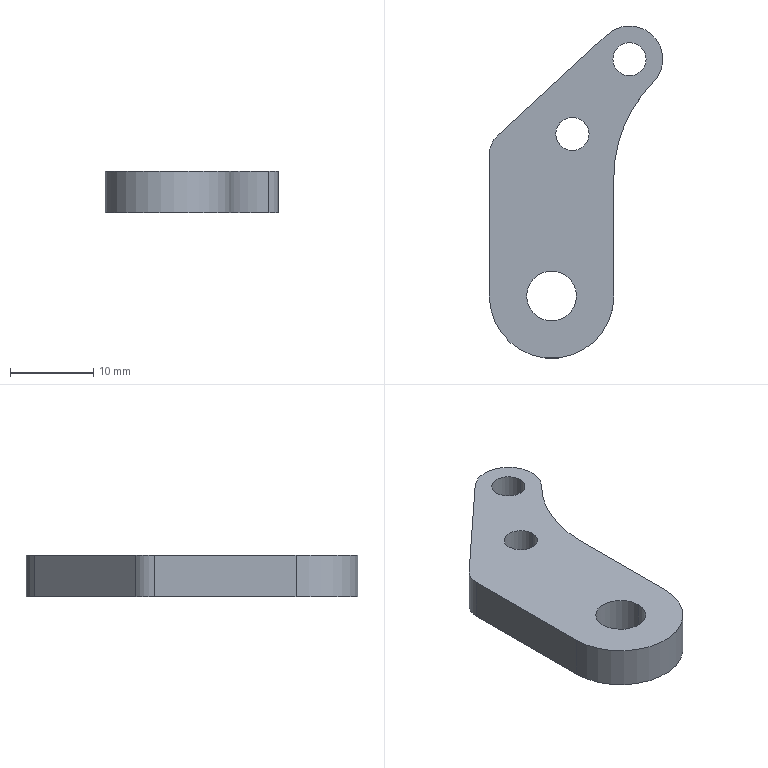Part | SolidWorks | features Extrusion 1 | 1 solid | 15 faces | box 20.88 x 40 x 5 mm | volume 2331 mm3 | cylinder 10 | plane 5 | commonest cylinder face diameters 4 x4 6 x3 8 x1 15 x1 32 x1
STEP:
#1=CARTESIAN_POINT('',(7.38,28.5,5.));
#2=VERTEX_POINT('',#1);
#3=CARTESIAN_POINT('',(11.38,28.5,5.));
#4=VERTEX_POINT('',#3);
#5=CARTESIAN_POINT('',(9.38,28.5,5.));
#6=DIRECTION('',(0.,0.,1.));
#7=DIRECTION('',(1.,0.,0.));
#8=AXIS2_PLACEMENT_3D('',#5,#6,#7);
#9=CIRCLE('',#8,2.);
#10=EDGE_CURVE('',#2,#4,#9,.T.);
#11=ORIENTED_EDGE('',*,*,#10,.T.);
#12=CARTESIAN_POINT('',(11.38,28.5,0.));
#13=VERTEX_POINT('',#12);
#14=CARTESIAN_POINT('',(11.38,28.5,5.));
#15=DIRECTION('',(0.,0.,-1.));
#16=VECTOR('',#15,1000.);
#17=LINE('',#14,#16);
#18=EDGE_CURVE('',#4,#13,#17,.T.);
#19=ORIENTED_EDGE('',*,*,#18,.T.);
#20=CARTESIAN_POINT('',(7.38,28.5,0.));
#21=VERTEX_POINT('',#20);
#22=CARTESIAN_POINT('',(9.38,28.5,0.));
#23=DIRECTION('',(0.,0.,1.));
#24=DIRECTION('',(1.,0.,0.));
#25=AXIS2_PLACEMENT_3D('',#22,#23,#24);
#26=CIRCLE('',#25,2.);
#27=EDGE_CURVE('',#21,#13,#26,.T.);
#28=ORIENTED_EDGE('',*,*,#27,.F.);
#29=CARTESIAN_POINT('',(7.38,28.5,5.));
#30=DIRECTION('',(0.,0.,-1.));
#31=VECTOR('',#30,1000.);
#32=LINE('',#29,#31);
#33=EDGE_CURVE('',#2,#21,#32,.T.);
#34=ORIENTED_EDGE('',*,*,#33,.F.);
#35=EDGE_LOOP('',(#11,#19,#28,#34));
#36=FACE_OUTER_BOUND('',#35,.T.);
#37=CARTESIAN_POINT('',(9.38,28.5,5.));
#38=DIRECTION('',(0.,0.,-1.));
#39=DIRECTION('',(-1.,0.,0.));
#40=AXIS2_PLACEMENT_3D('',#37,#38,#39);
#41=CYLINDRICAL_SURFACE('',#40,2.);
#42=ADVANCED_FACE('',(#36),#41,.F.);
#43=CARTESIAN_POINT('',(0.5,19.5,5.));
#44=VERTEX_POINT('',#43);
#45=CARTESIAN_POINT('',(4.5,19.5,5.));
#46=VERTEX_POINT('',#45);
#47=CARTESIAN_POINT('',(2.5,19.5,5.));
#48=DIRECTION('',(0.,0.,1.));
#49=DIRECTION('',(1.,0.,0.));
#50=AXIS2_PLACEMENT_3D('',#47,#48,#49);
#51=CIRCLE('',#50,2.);
#52=EDGE_CURVE('',#44,#46,#51,.T.);
#53=ORIENTED_EDGE('',*,*,#52,.T.);
#54=CARTESIAN_POINT('',(4.5,19.5,0.));
#55=VERTEX_POINT('',#54);
#56=CARTESIAN_POINT('',(4.5,19.5,5.));
#57=DIRECTION('',(0.,0.,-1.));
#58=VECTOR('',#57,1000.);
#59=LINE('',#56,#58);
#60=EDGE_CURVE('',#46,#55,#59,.T.);
#61=ORIENTED_EDGE('',*,*,#60,.T.);
#62=CARTESIAN_POINT('',(0.5,19.5,0.));
#63=VERTEX_POINT('',#62);
#64=CARTESIAN_POINT('',(2.5,19.5,0.));
#65=DIRECTION('',(0.,0.,1.));
#66=DIRECTION('',(1.,0.,0.));
#67=AXIS2_PLACEMENT_3D('',#64,#65,#66);
#68=CIRCLE('',#67,2.);
#69=EDGE_CURVE('',#63,#55,#68,.T.);
#70=ORIENTED_EDGE('',*,*,#69,.F.);
#71=CARTESIAN_POINT('',(0.5,19.5,5.));
#72=DIRECTION('',(0.,0.,-1.));
#73=VECTOR('',#72,1000.);
#74=LINE('',#71,#73);
#75=EDGE_CURVE('',#44,#63,#74,.T.);
#76=ORIENTED_EDGE('',*,*,#75,.F.);
#77=EDGE_LOOP('',(#53,#61,#70,#76));
#78=FACE_OUTER_BOUND('',#77,.T.);
#79=CARTESIAN_POINT('',(2.5,19.5,5.));
#80=DIRECTION('',(0.,0.,-1.));
#81=DIRECTION('',(-1.,0.,0.));
#82=AXIS2_PLACEMENT_3D('',#79,#80,#81);
#83=CYLINDRICAL_SURFACE('',#82,2.);
#84=ADVANCED_FACE('',(#78),#83,.F.);
#85=CARTESIAN_POINT('',(-3.,0.,5.));
#86=VERTEX_POINT('',#85);
#87=CARTESIAN_POINT('',(3.,0.,5.));
#88=VERTEX_POINT('',#87);
#89=CARTESIAN_POINT('',(0.,0.,5.));
#90=DIRECTION('',(0.,0.,1.));
#91=DIRECTION('',(1.,0.,0.));
#92=AXIS2_PLACEMENT_3D('',#89,#90,#91);
#93=CIRCLE('',#92,3.);
#94=EDGE_CURVE('',#86,#88,#93,.T.);
#95=ORIENTED_EDGE('',*,*,#94,.T.);
#96=CARTESIAN_POINT('',(3.,0.,0.));
#97=VERTEX_POINT('',#96);
#98=CARTESIAN_POINT('',(3.,0.,5.));
#99=DIRECTION('',(0.,0.,-1.));
#100=VECTOR('',#99,1000.);
#101=LINE('',#98,#100);
#102=EDGE_CURVE('',#88,#97,#101,.T.);
#103=ORIENTED_EDGE('',*,*,#102,.T.);
#104=CARTESIAN_POINT('',(-3.,0.,0.));
#105=VERTEX_POINT('',#104);
#106=CARTESIAN_POINT('',(0.,0.,0.));
#107=DIRECTION('',(0.,0.,1.));
#108=DIRECTION('',(1.,0.,0.));
#109=AXIS2_PLACEMENT_3D('',#106,#107,#108);
#110=CIRCLE('',#109,3.);
#111=EDGE_CURVE('',#105,#97,#110,.T.);
#112=ORIENTED_EDGE('',*,*,#111,.F.);
#113=CARTESIAN_POINT('',(-3.,0.,5.));
#114=DIRECTION('',(0.,0.,-1.));
#115=VECTOR('',#114,1000.);
#116=LINE('',#113,#115);
#117=EDGE_CURVE('',#86,#105,#116,.T.);
#118=ORIENTED_EDGE('',*,*,#117,.F.);
#119=EDGE_LOOP('',(#95,#103,#112,#118));
#120=FACE_OUTER_BOUND('',#119,.T.);
#121=CARTESIAN_POINT('',(0.,0.,5.));
#122=DIRECTION('',(0.,0.,-1.));
#123=DIRECTION('',(-1.,0.,0.));
#124=AXIS2_PLACEMENT_3D('',#121,#122,#123);
#125=CYLINDRICAL_SURFACE('',#124,3.);
#126=ADVANCED_FACE('',(#120),#125,.F.);
#127=ORIENTED_EDGE('',*,*,#52,.F.);
#128=CARTESIAN_POINT('',(2.5,19.5,5.));
#129=DIRECTION('',(0.,0.,1.));
#130=DIRECTION('',(1.,0.,0.));
#131=AXIS2_PLACEMENT_3D('',#128,#129,#130);
#132=CIRCLE('',#131,2.);
#133=EDGE_CURVE('',#46,#44,#132,.T.);
#134=ORIENTED_EDGE('',*,*,#133,.F.);
#135=EDGE_LOOP('',(#127,#134));
#136=FACE_BOUND('',#135,.T.);
#137=CARTESIAN_POINT('',(-6.533,19.28,5.));
#138=VERTEX_POINT('',#137);
#139=CARTESIAN_POINT('',(-7.5,17.074,5.));
#140=VERTEX_POINT('',#139);
#141=CARTESIAN_POINT('',(-4.5,17.074,5.));
#142=DIRECTION('',(0.,0.,1.));
#143=DIRECTION('',(1.,0.,0.));
#144=AXIS2_PLACEMENT_3D('',#141,#142,#143);
#145=CIRCLE('',#144,3.);
#146=EDGE_CURVE('',#138,#140,#145,.T.);
#147=ORIENTED_EDGE('',*,*,#146,.T.);
#148=CARTESIAN_POINT('',(-7.5,0.,5.));
#149=VERTEX_POINT('',#148);
#150=CARTESIAN_POINT('',(-7.5,0.,5.));
#151=DIRECTION('',(0.,-1.,0.));
#152=VECTOR('',#151,1000.);
#153=LINE('',#150,#152);
#154=EDGE_CURVE('',#140,#149,#153,.T.);
#155=ORIENTED_EDGE('',*,*,#154,.T.);
#156=CARTESIAN_POINT('',(7.5,0.,5.));
#157=VERTEX_POINT('',#156);
#158=CARTESIAN_POINT('',(0.,0.,5.));
#159=DIRECTION('',(0.,0.,1.));
#160=DIRECTION('',(1.,0.,0.));
#161=AXIS2_PLACEMENT_3D('',#158,#159,#160);
#162=CIRCLE('',#161,7.5);
#163=EDGE_CURVE('',#149,#157,#162,.T.);
#164=ORIENTED_EDGE('',*,*,#163,.T.);
#165=CARTESIAN_POINT('',(7.5,14.336,5.));
#166=VERTEX_POINT('',#165);
#167=CARTESIAN_POINT('',(7.5,0.,5.));
#168=DIRECTION('',(0.,1.,0.));
#169=VECTOR('',#168,1000.);
#170=LINE('',#167,#169);
#171=EDGE_CURVE('',#157,#166,#170,.T.);
#172=ORIENTED_EDGE('',*,*,#171,.T.);
#173=CARTESIAN_POINT('',(12.204,25.667,5.));
#174=VERTEX_POINT('',#173);
#175=CARTESIAN_POINT('',(23.5,14.336,5.));
#176=DIRECTION('',(0.,0.,-1.));
#177=DIRECTION('',(1.,0.,0.));
#178=AXIS2_PLACEMENT_3D('',#175,#176,#177);
#179=CIRCLE('',#178,16.);
#180=EDGE_CURVE('',#166,#174,#179,.T.);
#181=ORIENTED_EDGE('',*,*,#180,.T.);
#182=CARTESIAN_POINT('',(6.67,31.442,5.));
#183=VERTEX_POINT('',#182);
#184=CARTESIAN_POINT('',(9.38,28.5,5.));
#185=DIRECTION('',(0.,0.,1.));
#186=DIRECTION('',(1.,0.,0.));
#187=AXIS2_PLACEMENT_3D('',#184,#185,#186);
#188=CIRCLE('',#187,4.);
#189=EDGE_CURVE('',#174,#183,#188,.T.);
#190=ORIENTED_EDGE('',*,*,#189,.T.);
#191=CARTESIAN_POINT('',(-6.533,19.28,5.));
#192=DIRECTION('',(-0.7355,-0.6775,0.));
#193=VECTOR('',#192,1000.);
#194=LINE('',#191,#193);
#195=EDGE_CURVE('',#183,#138,#194,.T.);
#196=ORIENTED_EDGE('',*,*,#195,.T.);
#197=EDGE_LOOP('',(#147,#155,#164,#172,#181,#190,#196));
#198=FACE_OUTER_BOUND('',#197,.T.);
#199=ORIENTED_EDGE('',*,*,#94,.F.);
#200=CARTESIAN_POINT('',(0.,0.,5.));
#201=DIRECTION('',(0.,0.,1.));
#202=DIRECTION('',(1.,0.,0.));
#203=AXIS2_PLACEMENT_3D('',#200,#201,#202);
#204=CIRCLE('',#203,3.);
#205=EDGE_CURVE('',#88,#86,#204,.T.);
#206=ORIENTED_EDGE('',*,*,#205,.F.);
#207=EDGE_LOOP('',(#199,#206));
#208=FACE_BOUND('',#207,.T.);
#209=ORIENTED_EDGE('',*,*,#10,.F.);
#210=CARTESIAN_POINT('',(9.38,28.5,5.));
#211=DIRECTION('',(0.,0.,1.));
#212=DIRECTION('',(1.,0.,0.));
#213=AXIS2_PLACEMENT_3D('',#210,#211,#212);
#214=CIRCLE('',#213,2.);
#215=EDGE_CURVE('',#4,#2,#214,.T.);
#216=ORIENTED_EDGE('',*,*,#215,.F.);
#217=EDGE_LOOP('',(#209,#216));
#218=FACE_BOUND('',#217,.T.);
#219=CARTESIAN_POINT('',(-4.5,17.074,5.));
#220=DIRECTION('',(0.,0.,1.));
#221=DIRECTION('',(1.,0.,0.));
#222=AXIS2_PLACEMENT_3D('',#219,#220,#221);
#223=PLANE('',#222);
#224=ADVANCED_FACE('',(#136,#198,#208,#218),#223,.T.);
#225=CARTESIAN_POINT('',(-6.533,19.28,0.));
#226=VERTEX_POINT('',#225);
#227=CARTESIAN_POINT('',(-7.5,17.074,0.));
#228=VERTEX_POINT('',#227);
#229=CARTESIAN_POINT('',(-4.5,17.074,0.));
#230=DIRECTION('',(0.,0.,1.));
#231=DIRECTION('',(1.,0.,0.));
#232=AXIS2_PLACEMENT_3D('',#229,#230,#231);
#233=CIRCLE('',#232,3.);
#234=EDGE_CURVE('',#226,#228,#233,.T.);
#235=ORIENTED_EDGE('',*,*,#234,.F.);
#236=CARTESIAN_POINT('',(6.67,31.442,0.));
#237=VERTEX_POINT('',#236);
#238=CARTESIAN_POINT('',(-6.533,19.28,0.));
#239=DIRECTION('',(-0.7355,-0.6775,0.));
#240=VECTOR('',#239,1000.);
#241=LINE('',#238,#240);
#242=EDGE_CURVE('',#237,#226,#241,.T.);
#243=ORIENTED_EDGE('',*,*,#242,.F.);
#244=CARTESIAN_POINT('',(12.204,25.667,0.));
#245=VERTEX_POINT('',#244);
#246=CARTESIAN_POINT('',(9.38,28.5,0.));
#247=DIRECTION('',(0.,0.,1.));
#248=DIRECTION('',(1.,0.,0.));
#249=AXIS2_PLACEMENT_3D('',#246,#247,#248);
#250=CIRCLE('',#249,4.);
#251=EDGE_CURVE('',#245,#237,#250,.T.);
#252=ORIENTED_EDGE('',*,*,#251,.F.);
#253=CARTESIAN_POINT('',(7.5,14.336,0.));
#254=VERTEX_POINT('',#253);
#255=CARTESIAN_POINT('',(23.5,14.336,0.));
#256=DIRECTION('',(0.,0.,-1.));
#257=DIRECTION('',(1.,0.,0.));
#258=AXIS2_PLACEMENT_3D('',#255,#256,#257);
#259=CIRCLE('',#258,16.);
#260=EDGE_CURVE('',#254,#245,#259,.T.);
#261=ORIENTED_EDGE('',*,*,#260,.F.);
#262=CARTESIAN_POINT('',(7.5,0.,0.));
#263=VERTEX_POINT('',#262);
#264=CARTESIAN_POINT('',(7.5,0.,0.));
#265=DIRECTION('',(0.,1.,0.));
#266=VECTOR('',#265,1000.);
#267=LINE('',#264,#266);
#268=EDGE_CURVE('',#263,#254,#267,.T.);
#269=ORIENTED_EDGE('',*,*,#268,.F.);
#270=CARTESIAN_POINT('',(-7.5,0.,0.));
#271=VERTEX_POINT('',#270);
#272=CARTESIAN_POINT('',(0.,0.,0.));
#273=DIRECTION('',(0.,0.,1.));
#274=DIRECTION('',(1.,0.,0.));
#275=AXIS2_PLACEMENT_3D('',#272,#273,#274);
#276=CIRCLE('',#275,7.5);
#277=EDGE_CURVE('',#271,#263,#276,.T.);
#278=ORIENTED_EDGE('',*,*,#277,.F.);
#279=CARTESIAN_POINT('',(-7.5,0.,0.));
#280=DIRECTION('',(0.,-1.,0.));
#281=VECTOR('',#280,1000.);
#282=LINE('',#279,#281);
#283=EDGE_CURVE('',#228,#271,#282,.T.);
#284=ORIENTED_EDGE('',*,*,#283,.F.);
#285=EDGE_LOOP('',(#235,#243,#252,#261,#269,#278,#284));
#286=FACE_OUTER_BOUND('',#285,.T.);
#287=ORIENTED_EDGE('',*,*,#111,.T.);
#288=CARTESIAN_POINT('',(0.,0.,0.));
#289=DIRECTION('',(0.,0.,1.));
#290=DIRECTION('',(1.,0.,0.));
#291=AXIS2_PLACEMENT_3D('',#288,#289,#290);
#292=CIRCLE('',#291,3.);
#293=EDGE_CURVE('',#97,#105,#292,.T.);
#294=ORIENTED_EDGE('',*,*,#293,.T.);
#295=EDGE_LOOP('',(#287,#294));
#296=FACE_BOUND('',#295,.T.);
#297=ORIENTED_EDGE('',*,*,#69,.T.);
#298=CARTESIAN_POINT('',(2.5,19.5,0.));
#299=DIRECTION('',(0.,0.,1.));
#300=DIRECTION('',(1.,0.,0.));
#301=AXIS2_PLACEMENT_3D('',#298,#299,#300);
#302=CIRCLE('',#301,2.);
#303=EDGE_CURVE('',#55,#63,#302,.T.);
#304=ORIENTED_EDGE('',*,*,#303,.T.);
#305=EDGE_LOOP('',(#297,#304));
#306=FACE_BOUND('',#305,.T.);
#307=ORIENTED_EDGE('',*,*,#27,.T.);
#308=CARTESIAN_POINT('',(9.38,28.5,0.));
#309=DIRECTION('',(0.,0.,1.));
#310=DIRECTION('',(1.,0.,0.));
#311=AXIS2_PLACEMENT_3D('',#308,#309,#310);
#312=CIRCLE('',#311,2.);
#313=EDGE_CURVE('',#13,#21,#312,.T.);
#314=ORIENTED_EDGE('',*,*,#313,.T.);
#315=EDGE_LOOP('',(#307,#314));
#316=FACE_BOUND('',#315,.T.);
#317=CARTESIAN_POINT('',(-4.5,17.074,0.));
#318=DIRECTION('',(0.,0.,1.));
#319=DIRECTION('',(1.,0.,0.));
#320=AXIS2_PLACEMENT_3D('',#317,#318,#319);
#321=PLANE('',#320);
#322=ADVANCED_FACE('',(#286,#296,#306,#316),#321,.F.);
#323=ORIENTED_EDGE('',*,*,#234,.T.);
#324=CARTESIAN_POINT('',(-7.5,17.074,5.));
#325=DIRECTION('',(0.,0.,-1.));
#326=VECTOR('',#325,1000.);
#327=LINE('',#324,#326);
#328=EDGE_CURVE('',#140,#228,#327,.T.);
#329=ORIENTED_EDGE('',*,*,#328,.F.);
#330=ORIENTED_EDGE('',*,*,#146,.F.);
#331=CARTESIAN_POINT('',(-6.533,19.28,5.));
#332=DIRECTION('',(0.,0.,-1.));
#333=VECTOR('',#332,1000.);
#334=LINE('',#331,#333);
#335=EDGE_CURVE('',#138,#226,#334,.T.);
#336=ORIENTED_EDGE('',*,*,#335,.T.);
#337=EDGE_LOOP('',(#323,#329,#330,#336));
#338=FACE_OUTER_BOUND('',#337,.T.);
#339=CARTESIAN_POINT('',(-4.5,17.074,5.));
#340=DIRECTION('',(0.,0.,-1.));
#341=DIRECTION('',(-1.,0.,0.));
#342=AXIS2_PLACEMENT_3D('',#339,#340,#341);
#343=CYLINDRICAL_SURFACE('',#342,3.);
#344=ADVANCED_FACE('',(#338),#343,.T.);
#345=ORIENTED_EDGE('',*,*,#283,.T.);
#346=CARTESIAN_POINT('',(-7.5,0.,5.));
#347=DIRECTION('',(0.,0.,-1.));
#348=VECTOR('',#347,1000.);
#349=LINE('',#346,#348);
#350=EDGE_CURVE('',#149,#271,#349,.T.);
#351=ORIENTED_EDGE('',*,*,#350,.F.);
#352=ORIENTED_EDGE('',*,*,#154,.F.);
#353=ORIENTED_EDGE('',*,*,#328,.T.);
#354=EDGE_LOOP('',(#345,#351,#352,#353));
#355=FACE_OUTER_BOUND('',#354,.T.);
#356=CARTESIAN_POINT('',(-7.5,0.,5.));
#357=DIRECTION('',(1.,0.,0.));
#358=DIRECTION('',(0.,0.,-1.));
#359=AXIS2_PLACEMENT_3D('',#356,#357,#358);
#360=PLANE('',#359);
#361=ADVANCED_FACE('',(#355),#360,.F.);
#362=ORIENTED_EDGE('',*,*,#277,.T.);
#363=CARTESIAN_POINT('',(7.5,0.,5.));
#364=DIRECTION('',(0.,0.,-1.));
#365=VECTOR('',#364,1000.);
#366=LINE('',#363,#365);
#367=EDGE_CURVE('',#157,#263,#366,.T.);
#368=ORIENTED_EDGE('',*,*,#367,.F.);
#369=ORIENTED_EDGE('',*,*,#163,.F.);
#370=ORIENTED_EDGE('',*,*,#350,.T.);
#371=EDGE_LOOP('',(#362,#368,#369,#370));
#372=FACE_OUTER_BOUND('',#371,.T.);
#373=CARTESIAN_POINT('',(0.,0.,5.));
#374=DIRECTION('',(0.,0.,-1.));
#375=DIRECTION('',(-1.,0.,0.));
#376=AXIS2_PLACEMENT_3D('',#373,#374,#375);
#377=CYLINDRICAL_SURFACE('',#376,7.5);
#378=ADVANCED_FACE('',(#372),#377,.T.);
#379=ORIENTED_EDGE('',*,*,#268,.T.);
#380=CARTESIAN_POINT('',(7.5,14.336,5.));
#381=DIRECTION('',(0.,0.,-1.));
#382=VECTOR('',#381,1000.);
#383=LINE('',#380,#382);
#384=EDGE_CURVE('',#166,#254,#383,.T.);
#385=ORIENTED_EDGE('',*,*,#384,.F.);
#386=ORIENTED_EDGE('',*,*,#171,.F.);
#387=ORIENTED_EDGE('',*,*,#367,.T.);
#388=EDGE_LOOP('',(#379,#385,#386,#387));
#389=FACE_OUTER_BOUND('',#388,.T.);
#390=CARTESIAN_POINT('',(7.5,0.,5.));
#391=DIRECTION('',(-1.,0.,0.));
#392=DIRECTION('',(0.,0.,1.));
#393=AXIS2_PLACEMENT_3D('',#390,#391,#392);
#394=PLANE('',#393);
#395=ADVANCED_FACE('',(#389),#394,.F.);
#396=ORIENTED_EDGE('',*,*,#260,.T.);
#397=CARTESIAN_POINT('',(12.204,25.667,5.));
#398=DIRECTION('',(0.,0.,-1.));
#399=VECTOR('',#398,1000.);
#400=LINE('',#397,#399);
#401=EDGE_CURVE('',#174,#245,#400,.T.);
#402=ORIENTED_EDGE('',*,*,#401,.F.);
#403=ORIENTED_EDGE('',*,*,#180,.F.);
#404=ORIENTED_EDGE('',*,*,#384,.T.);
#405=EDGE_LOOP('',(#396,#402,#403,#404));
#406=FACE_OUTER_BOUND('',#405,.T.);
#407=CARTESIAN_POINT('',(23.5,14.336,5.));
#408=DIRECTION('',(0.,0.,-1.));
#409=DIRECTION('',(-1.,0.,0.));
#410=AXIS2_PLACEMENT_3D('',#407,#408,#409);
#411=CYLINDRICAL_SURFACE('',#410,16.);
#412=ADVANCED_FACE('',(#406),#411,.F.);
#413=ORIENTED_EDGE('',*,*,#251,.T.);
#414=CARTESIAN_POINT('',(6.67,31.442,5.));
#415=DIRECTION('',(0.,0.,-1.));
#416=VECTOR('',#415,1000.);
#417=LINE('',#414,#416);
#418=EDGE_CURVE('',#183,#237,#417,.T.);
#419=ORIENTED_EDGE('',*,*,#418,.F.);
#420=ORIENTED_EDGE('',*,*,#189,.F.);
#421=ORIENTED_EDGE('',*,*,#401,.T.);
#422=EDGE_LOOP('',(#413,#419,#420,#421));
#423=FACE_OUTER_BOUND('',#422,.T.);
#424=CARTESIAN_POINT('',(9.38,28.5,5.));
#425=DIRECTION('',(0.,0.,-1.));
#426=DIRECTION('',(-1.,0.,0.));
#427=AXIS2_PLACEMENT_3D('',#424,#425,#426);
#428=CYLINDRICAL_SURFACE('',#427,4.);
#429=ADVANCED_FACE('',(#423),#428,.T.);
#430=ORIENTED_EDGE('',*,*,#242,.T.);
#431=ORIENTED_EDGE('',*,*,#335,.F.);
#432=ORIENTED_EDGE('',*,*,#195,.F.);
#433=ORIENTED_EDGE('',*,*,#418,.T.);
#434=EDGE_LOOP('',(#430,#431,#432,#433));
#435=FACE_OUTER_BOUND('',#434,.T.);
#436=CARTESIAN_POINT('',(-6.533,19.28,5.));
#437=DIRECTION('',(0.6775,-0.7355,0.));
#438=DIRECTION('',(0.7355,0.6775,0.));
#439=AXIS2_PLACEMENT_3D('',#436,#437,#438);
#440=PLANE('',#439);
#441=ADVANCED_FACE('',(#435),#440,.F.);
#442=ORIENTED_EDGE('',*,*,#102,.F.);
#443=ORIENTED_EDGE('',*,*,#205,.T.);
#444=ORIENTED_EDGE('',*,*,#117,.T.);
#445=ORIENTED_EDGE('',*,*,#293,.F.);
#446=EDGE_LOOP('',(#442,#443,#444,#445));
#447=FACE_OUTER_BOUND('',#446,.T.);
#448=CARTESIAN_POINT('',(0.,0.,5.));
#449=DIRECTION('',(0.,0.,-1.));
#450=DIRECTION('',(-1.,0.,0.));
#451=AXIS2_PLACEMENT_3D('',#448,#449,#450);
#452=CYLINDRICAL_SURFACE('',#451,3.);
#453=ADVANCED_FACE('',(#447),#452,.F.);
#454=ORIENTED_EDGE('',*,*,#60,.F.);
#455=ORIENTED_EDGE('',*,*,#133,.T.);
#456=ORIENTED_EDGE('',*,*,#75,.T.);
#457=ORIENTED_EDGE('',*,*,#303,.F.);
#458=EDGE_LOOP('',(#454,#455,#456,#457));
#459=FACE_OUTER_BOUND('',#458,.T.);
#460=CARTESIAN_POINT('',(2.5,19.5,5.));
#461=DIRECTION('',(0.,0.,-1.));
#462=DIRECTION('',(-1.,0.,0.));
#463=AXIS2_PLACEMENT_3D('',#460,#461,#462);
#464=CYLINDRICAL_SURFACE('',#463,2.);
#465=ADVANCED_FACE('',(#459),#464,.F.);
#466=ORIENTED_EDGE('',*,*,#18,.F.);
#467=ORIENTED_EDGE('',*,*,#215,.T.);
#468=ORIENTED_EDGE('',*,*,#33,.T.);
#469=ORIENTED_EDGE('',*,*,#313,.F.);
#470=EDGE_LOOP('',(#466,#467,#468,#469));
#471=FACE_OUTER_BOUND('',#470,.T.);
#472=CARTESIAN_POINT('',(9.38,28.5,5.));
#473=DIRECTION('',(0.,0.,-1.));
#474=DIRECTION('',(-1.,0.,0.));
#475=AXIS2_PLACEMENT_3D('',#472,#473,#474);
#476=CYLINDRICAL_SURFACE('',#475,2.);
#477=ADVANCED_FACE('',(#471),#476,.F.);
#478=CLOSED_SHELL('',(#42,#84,#126,#224,#322,#344,#361,#378,#395,#412,#429,#441,#453,#465,#477));
#479=MANIFOLD_SOLID_BREP('',#478);
#480=CARTESIAN_POINT('',(0.,0.,0.));
#481=DIRECTION('',(0.,0.,1.));
#482=DIRECTION('',(1.,0.,0.));
#483=AXIS2_PLACEMENT_3D('',#480,#481,#482);
#484=(LENGTH_UNIT()NAMED_UNIT(*)SI_UNIT(.MILLI.,.METRE.));
#485=UNCERTAINTY_MEASURE_WITH_UNIT(LENGTH_MEASURE(0.00001),#484,'','');
#486=(NAMED_UNIT(*)PLANE_ANGLE_UNIT()SI_UNIT($,.RADIAN.));
#487=(NAMED_UNIT(*)SI_UNIT($,.STERADIAN.)SOLID_ANGLE_UNIT());
#488=(GEOMETRIC_REPRESENTATION_CONTEXT(3)GLOBAL_UNCERTAINTY_ASSIGNED_CONTEXT((#485))GLOBAL_UNIT_ASSIGNED_CONTEXT((#484,#486,#487))REPRESENTATION_CONTEXT('',''));
#489=ADVANCED_BREP_SHAPE_REPRESENTATION('',(#479,#483),#488);